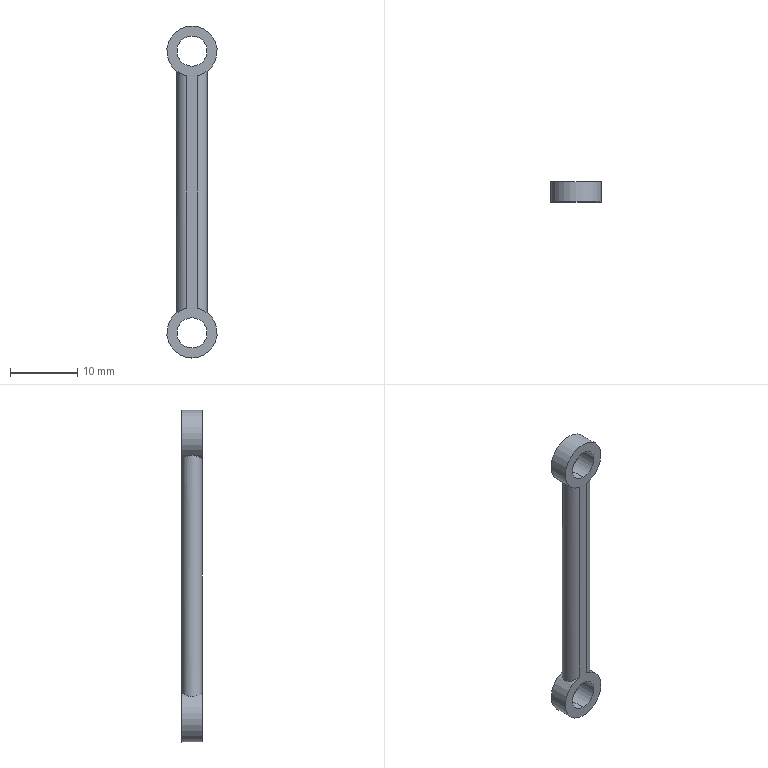Part | SolidWorks | features BaseBody 1, HoleWzd 1, Scale 1 | 1 solid | 12 faces | box 7.5 x 3 x 49.5 mm | volume 573.12 mm3 | cylinder 10 | plane 2 | commonest cylinder face diameters 4.5 x4 3 x3 7.5 x3
STEP:
#1=CARTESIAN_POINT('',(2.25,3.,44.25));
#2=VERTEX_POINT('',#1);
#3=CARTESIAN_POINT('',(2.25,3.,39.75));
#4=VERTEX_POINT('',#3);
#5=CARTESIAN_POINT('',(2.25,3.,42.));
#6=DIRECTION('',(0.,-1.,0.));
#7=DIRECTION('',(0.,0.,-1.));
#8=AXIS2_PLACEMENT_3D('',#5,#6,#7);
#9=CIRCLE('',#8,2.25);
#10=EDGE_CURVE('',#2,#4,#9,.T.);
#11=ORIENTED_EDGE('',*,*,#10,.F.);
#12=CARTESIAN_POINT('',(2.25,0.,44.25));
#13=VERTEX_POINT('',#12);
#14=CARTESIAN_POINT('',(2.25,0.,44.25));
#15=DIRECTION('',(0.,-1.,0.));
#16=VECTOR('',#15,1000.);
#17=LINE('',#14,#16);
#18=EDGE_CURVE('',#2,#13,#17,.T.);
#19=ORIENTED_EDGE('',*,*,#18,.T.);
#20=CARTESIAN_POINT('',(2.25,0.,39.75));
#21=VERTEX_POINT('',#20);
#22=CARTESIAN_POINT('',(2.25,0.,42.));
#23=DIRECTION('',(0.,-1.,0.));
#24=DIRECTION('',(0.,0.,-1.));
#25=AXIS2_PLACEMENT_3D('',#22,#23,#24);
#26=CIRCLE('',#25,2.25);
#27=EDGE_CURVE('',#13,#21,#26,.T.);
#28=ORIENTED_EDGE('',*,*,#27,.T.);
#29=CARTESIAN_POINT('',(2.25,0.,39.75));
#30=DIRECTION('',(0.,-1.,0.));
#31=VECTOR('',#30,1000.);
#32=LINE('',#29,#31);
#33=EDGE_CURVE('',#4,#21,#32,.T.);
#34=ORIENTED_EDGE('',*,*,#33,.F.);
#35=EDGE_LOOP('',(#11,#19,#28,#34));
#36=FACE_OUTER_BOUND('',#35,.T.);
#37=CARTESIAN_POINT('',(2.25,0.,42.));
#38=DIRECTION('',(0.,-1.,0.));
#39=DIRECTION('',(0.,0.,-1.));
#40=AXIS2_PLACEMENT_3D('',#37,#38,#39);
#41=CYLINDRICAL_SURFACE('',#40,2.25);
#42=ADVANCED_FACE('',(#36),#41,.F.);
#43=CARTESIAN_POINT('',(2.25,3.,2.25));
#44=VERTEX_POINT('',#43);
#45=CARTESIAN_POINT('',(2.25,3.,-2.25));
#46=VERTEX_POINT('',#45);
#47=CARTESIAN_POINT('',(2.25,3.,0.));
#48=DIRECTION('',(0.,-1.,0.));
#49=DIRECTION('',(0.,0.,-1.));
#50=AXIS2_PLACEMENT_3D('',#47,#48,#49);
#51=CIRCLE('',#50,2.25);
#52=EDGE_CURVE('',#44,#46,#51,.T.);
#53=ORIENTED_EDGE('',*,*,#52,.F.);
#54=CARTESIAN_POINT('',(2.25,0.,2.25));
#55=VERTEX_POINT('',#54);
#56=CARTESIAN_POINT('',(2.25,0.,2.25));
#57=DIRECTION('',(0.,-1.,0.));
#58=VECTOR('',#57,1000.);
#59=LINE('',#56,#58);
#60=EDGE_CURVE('',#44,#55,#59,.T.);
#61=ORIENTED_EDGE('',*,*,#60,.T.);
#62=CARTESIAN_POINT('',(2.25,0.,-2.25));
#63=VERTEX_POINT('',#62);
#64=CARTESIAN_POINT('',(2.25,0.,0.));
#65=DIRECTION('',(0.,-1.,0.));
#66=DIRECTION('',(0.,0.,-1.));
#67=AXIS2_PLACEMENT_3D('',#64,#65,#66);
#68=CIRCLE('',#67,2.25);
#69=EDGE_CURVE('',#55,#63,#68,.T.);
#70=ORIENTED_EDGE('',*,*,#69,.T.);
#71=CARTESIAN_POINT('',(2.25,0.,-2.25));
#72=DIRECTION('',(0.,-1.,0.));
#73=VECTOR('',#72,1000.);
#74=LINE('',#71,#73);
#75=EDGE_CURVE('',#46,#63,#74,.T.);
#76=ORIENTED_EDGE('',*,*,#75,.F.);
#77=EDGE_LOOP('',(#53,#61,#70,#76));
#78=FACE_OUTER_BOUND('',#77,.T.);
#79=CARTESIAN_POINT('',(2.25,0.,0.));
#80=DIRECTION('',(0.,-1.,0.));
#81=DIRECTION('',(0.,0.,-1.));
#82=AXIS2_PLACEMENT_3D('',#79,#80,#81);
#83=CYLINDRICAL_SURFACE('',#82,2.25);
#84=ADVANCED_FACE('',(#78),#83,.F.);
#85=CARTESIAN_POINT('',(3.,0.,3.674));
#86=VERTEX_POINT('',#85);
#87=CARTESIAN_POINT('',(4.5,1.5,3.));
#88=VERTEX_POINT('',#87);
#89=CARTESIAN_POINT('',(3.,0.,3.674));
#90=CARTESIAN_POINT('',(3.102,0.,3.654));
#91=CARTESIAN_POINT('',(3.2,0.0102,3.629));
#92=CARTESIAN_POINT('',(3.393,0.04905,3.573));
#93=CARTESIAN_POINT('',(3.488,0.07814,3.541));
#94=CARTESIAN_POINT('',(3.667,0.1528,3.473));
#95=CARTESIAN_POINT('',(3.751,0.1981,3.438));
#96=CARTESIAN_POINT('',(3.911,0.3041,3.363));
#97=CARTESIAN_POINT('',(3.986,0.3652,3.325));
#98=CARTESIAN_POINT('',(4.189,0.5659,3.213));
#99=CARTESIAN_POINT('',(4.301,0.728,3.141));
#100=CARTESIAN_POINT('',(4.418,1.,3.06));
#101=CARTESIAN_POINT('',(4.448,1.097,3.038));
#102=CARTESIAN_POINT('',(4.49,1.296,3.008));
#103=CARTESIAN_POINT('',(4.5,1.397,3.));
#104=CARTESIAN_POINT('',(4.5,1.5,3.));
#105=B_SPLINE_CURVE_WITH_KNOTS('',3,(#89,#90,#91,#92,#93,#94,#95,#96,#97,#98,#99,#100,#101,#102,#103,#104),.UNSPECIFIED.,.F.,.F.,(4,2,2,2,2,2,2,4),(0.,0.0003062,0.0006124,0.0009186,0.001225,0.001837,0.002143,0.00245),.UNSPECIFIED.);
#106=EDGE_CURVE('',#86,#88,#105,.T.);
#107=ORIENTED_EDGE('',*,*,#106,.T.);
#108=CARTESIAN_POINT('',(4.5,1.5,39.));
#109=VERTEX_POINT('',#108);
#110=CARTESIAN_POINT('',(4.5,1.5,0.));
#111=DIRECTION('',(0.,0.,1.));
#112=VECTOR('',#111,1000.);
#113=LINE('',#110,#112);
#114=EDGE_CURVE('',#88,#109,#113,.T.);
#115=ORIENTED_EDGE('',*,*,#114,.T.);
#116=CARTESIAN_POINT('',(3.,0.,38.326));
#117=VERTEX_POINT('',#116);
#118=CARTESIAN_POINT('',(4.5,1.5,39.));
#119=CARTESIAN_POINT('',(4.5,1.398,39.));
#120=CARTESIAN_POINT('',(4.489,1.294,38.992));
#121=CARTESIAN_POINT('',(4.448,1.096,38.962));
#122=CARTESIAN_POINT('',(4.417,0.9993,38.939));
#123=CARTESIAN_POINT('',(4.3,0.7262,38.859));
#124=CARTESIAN_POINT('',(4.188,0.5647,38.786));
#125=CARTESIAN_POINT('',(3.917,0.2975,38.637));
#126=CARTESIAN_POINT('',(3.755,0.1897,38.56));
#127=CARTESIAN_POINT('',(3.488,0.07846,38.459));
#128=CARTESIAN_POINT('',(3.394,0.04921,38.427));
#129=CARTESIAN_POINT('',(3.2,0.01017,38.371));
#130=CARTESIAN_POINT('',(3.101,0.,38.346));
#131=CARTESIAN_POINT('',(3.,0.,38.326));
#132=B_SPLINE_CURVE_WITH_KNOTS('',3,(#118,#119,#120,#121,#122,#123,#124,#125,#126,#127,#128,#129,#130,#131),.UNSPECIFIED.,.F.,.F.,(4,2,2,2,2,2,4),(0.00245,0.002755,0.00306,0.003671,0.004282,0.004588,0.004893),.UNSPECIFIED.);
#133=EDGE_CURVE('',#109,#117,#132,.T.);
#134=ORIENTED_EDGE('',*,*,#133,.T.);
#135=CARTESIAN_POINT('',(3.,0.,0.));
#136=DIRECTION('',(0.,0.,-1.));
#137=VECTOR('',#136,1000.);
#138=LINE('',#135,#137);
#139=EDGE_CURVE('',#117,#86,#138,.T.);
#140=ORIENTED_EDGE('',*,*,#139,.T.);
#141=EDGE_LOOP('',(#107,#115,#134,#140));
#142=FACE_OUTER_BOUND('',#141,.T.);
#143=CARTESIAN_POINT('',(3.,1.5,0.));
#144=DIRECTION('',(0.,0.,1.));
#145=DIRECTION('',(1.,0.,0.));
#146=AXIS2_PLACEMENT_3D('',#143,#144,#145);
#147=CYLINDRICAL_SURFACE('',#146,1.5);
#148=ADVANCED_FACE('',(#142),#147,.T.);
#149=CARTESIAN_POINT('',(1.5,3.,3.674));
#150=VERTEX_POINT('',#149);
#151=CARTESIAN_POINT('',(2.25,3.,-3.75));
#152=VERTEX_POINT('',#151);
#153=CARTESIAN_POINT('',(2.25,3.,0.));
#154=DIRECTION('',(0.,-1.,0.));
#155=DIRECTION('',(0.,0.,-1.));
#156=AXIS2_PLACEMENT_3D('',#153,#154,#155);
#157=CIRCLE('',#156,3.75);
#158=EDGE_CURVE('',#150,#152,#157,.T.);
#159=ORIENTED_EDGE('',*,*,#158,.T.);
#160=CARTESIAN_POINT('',(2.25,0.,-3.75));
#161=VERTEX_POINT('',#160);
#162=CARTESIAN_POINT('',(2.25,3.,-3.75));
#163=DIRECTION('',(0.,-1.,0.));
#164=VECTOR('',#163,1000.);
#165=LINE('',#162,#164);
#166=EDGE_CURVE('',#152,#161,#165,.T.);
#167=ORIENTED_EDGE('',*,*,#166,.T.);
#168=CARTESIAN_POINT('',(1.5,0.,3.674));
#169=VERTEX_POINT('',#168);
#170=CARTESIAN_POINT('',(2.25,0.,0.));
#171=DIRECTION('',(0.,1.,0.));
#172=DIRECTION('',(0.,0.,-1.));
#173=AXIS2_PLACEMENT_3D('',#170,#171,#172);
#174=CIRCLE('',#173,3.75);
#175=EDGE_CURVE('',#161,#169,#174,.T.);
#176=ORIENTED_EDGE('',*,*,#175,.T.);
#177=CARTESIAN_POINT('',(1.5,0.,3.674));
#178=CARTESIAN_POINT('',(1.399,0.,3.654));
#179=CARTESIAN_POINT('',(1.3,0.01018,3.629));
#180=CARTESIAN_POINT('',(1.108,0.04892,3.573));
#181=CARTESIAN_POINT('',(1.013,0.07794,3.541));
#182=CARTESIAN_POINT('',(0.834,0.1524,3.474));
#183=CARTESIAN_POINT('',(0.7497,0.1976,3.438));
#184=CARTESIAN_POINT('',(0.5905,0.3034,3.364));
#185=CARTESIAN_POINT('',(0.5154,0.3644,3.326));
#186=CARTESIAN_POINT('',(0.3121,0.5646,3.214));
#187=CARTESIAN_POINT('',(0.1999,0.7263,3.141));
#188=CARTESIAN_POINT('',(0.08309,0.9979,3.061));
#189=CARTESIAN_POINT('',(0.05223,1.095,3.039));
#190=CARTESIAN_POINT('',(0.0108,1.294,3.008));
#191=CARTESIAN_POINT('',(0.0002187,1.394,3.));
#192=CARTESIAN_POINT('',(-0.0002121,1.599,3.));
#193=CARTESIAN_POINT('',(0.01036,1.703,3.008));
#194=CARTESIAN_POINT('',(0.05114,1.901,3.038));
#195=CARTESIAN_POINT('',(0.08176,1.998,3.06));
#196=CARTESIAN_POINT('',(0.1988,2.272,3.141));
#197=CARTESIAN_POINT('',(0.3108,2.434,3.213));
#198=CARTESIAN_POINT('',(0.5824,2.702,3.362));
#199=CARTESIAN_POINT('',(0.744,2.81,3.44));
#200=CARTESIAN_POINT('',(1.011,2.921,3.541));
#201=CARTESIAN_POINT('',(1.106,2.951,3.573));
#202=CARTESIAN_POINT('',(1.299,2.99,3.629));
#203=CARTESIAN_POINT('',(1.398,3.,3.654));
#204=CARTESIAN_POINT('',(1.5,3.,3.674));
#205=B_SPLINE_CURVE_WITH_KNOTS('',3,(#177,#178,#179,#180,#181,#182,#183,#184,#185,#186,#187,#188,#189,#190,#191,#192,#193,#194,#195,#196,#197,#198,#199,#200,#201,#202,#203,#204),.UNSPECIFIED.,.F.,.F.,(4,2,2,2,2,2,2,2,2,2,2,2,2,4),(0.,0.0003058,0.0006116,0.0009174,0.001223,0.001835,0.002141,0.002446,0.002752,0.003058,0.00367,0.004281,0.004587,0.004893),.UNSPECIFIED.);
#206=EDGE_CURVE('',#169,#150,#205,.T.);
#207=ORIENTED_EDGE('',*,*,#206,.T.);
#208=EDGE_LOOP('',(#159,#167,#176,#207));
#209=FACE_OUTER_BOUND('',#208,.T.);
#210=CARTESIAN_POINT('',(2.25,3.,0.));
#211=DIRECTION('',(0.,-1.,0.));
#212=DIRECTION('',(0.,0.,-1.));
#213=AXIS2_PLACEMENT_3D('',#210,#211,#212);
#214=CYLINDRICAL_SURFACE('',#213,3.75);
#215=ADVANCED_FACE('',(#209),#214,.T.);
#216=ORIENTED_EDGE('',*,*,#114,.F.);
#217=CARTESIAN_POINT('',(3.,3.,3.674));
#218=VERTEX_POINT('',#217);
#219=CARTESIAN_POINT('',(4.5,1.5,3.));
#220=CARTESIAN_POINT('',(4.5,1.602,3.));
#221=CARTESIAN_POINT('',(4.489,1.706,3.008));
#222=CARTESIAN_POINT('',(4.448,1.904,3.038));
#223=CARTESIAN_POINT('',(4.417,2.001,3.061));
#224=CARTESIAN_POINT('',(4.3,2.274,3.141));
#225=CARTESIAN_POINT('',(4.188,2.435,3.214));
#226=CARTESIAN_POINT('',(3.917,2.703,3.363));
#227=CARTESIAN_POINT('',(3.755,2.81,3.44));
#228=CARTESIAN_POINT('',(3.488,2.922,3.541));
#229=CARTESIAN_POINT('',(3.394,2.951,3.573));
#230=CARTESIAN_POINT('',(3.2,2.99,3.629));
#231=CARTESIAN_POINT('',(3.101,3.,3.654));
#232=CARTESIAN_POINT('',(3.,3.,3.674));
#233=B_SPLINE_CURVE_WITH_KNOTS('',3,(#219,#220,#221,#222,#223,#224,#225,#226,#227,#228,#229,#230,#231,#232),.UNSPECIFIED.,.F.,.F.,(4,2,2,2,2,2,4),(0.00245,0.002755,0.00306,0.003671,0.004282,0.004588,0.004893),.UNSPECIFIED.);
#234=EDGE_CURVE('',#88,#218,#233,.T.);
#235=ORIENTED_EDGE('',*,*,#234,.T.);
#236=CARTESIAN_POINT('',(3.,3.,38.326));
#237=VERTEX_POINT('',#236);
#238=CARTESIAN_POINT('',(3.,3.,0.));
#239=DIRECTION('',(0.,0.,1.));
#240=VECTOR('',#239,1000.);
#241=LINE('',#238,#240);
#242=EDGE_CURVE('',#218,#237,#241,.T.);
#243=ORIENTED_EDGE('',*,*,#242,.T.);
#244=CARTESIAN_POINT('',(3.,3.,38.326));
#245=CARTESIAN_POINT('',(3.102,3.,38.346));
#246=CARTESIAN_POINT('',(3.2,2.99,38.371));
#247=CARTESIAN_POINT('',(3.393,2.951,38.427));
#248=CARTESIAN_POINT('',(3.488,2.922,38.459));
#249=CARTESIAN_POINT('',(3.667,2.847,38.527));
#250=CARTESIAN_POINT('',(3.751,2.802,38.562));
#251=CARTESIAN_POINT('',(3.911,2.696,38.637));
#252=CARTESIAN_POINT('',(3.986,2.635,38.675));
#253=CARTESIAN_POINT('',(4.189,2.434,38.787));
#254=CARTESIAN_POINT('',(4.301,2.272,38.859));
#255=CARTESIAN_POINT('',(4.418,2.,38.94));
#256=CARTESIAN_POINT('',(4.448,1.903,38.962));
#257=CARTESIAN_POINT('',(4.49,1.704,38.992));
#258=CARTESIAN_POINT('',(4.5,1.603,39.));
#259=CARTESIAN_POINT('',(4.5,1.5,39.));
#260=B_SPLINE_CURVE_WITH_KNOTS('',3,(#244,#245,#246,#247,#248,#249,#250,#251,#252,#253,#254,#255,#256,#257,#258,#259),.UNSPECIFIED.,.F.,.F.,(4,2,2,2,2,2,2,4),(0.,0.0003062,0.0006124,0.0009186,0.001225,0.001837,0.002143,0.00245),.UNSPECIFIED.);
#261=EDGE_CURVE('',#237,#109,#260,.T.);
#262=ORIENTED_EDGE('',*,*,#261,.T.);
#263=EDGE_LOOP('',(#216,#235,#243,#262));
#264=FACE_OUTER_BOUND('',#263,.T.);
#265=CARTESIAN_POINT('',(3.,1.5,0.));
#266=DIRECTION('',(0.,0.,1.));
#267=DIRECTION('',(1.,0.,0.));
#268=AXIS2_PLACEMENT_3D('',#265,#266,#267);
#269=CYLINDRICAL_SURFACE('',#268,1.5);
#270=ADVANCED_FACE('',(#264),#269,.T.);
#271=ORIENTED_EDGE('',*,*,#166,.F.);
#272=CARTESIAN_POINT('',(2.25,3.,0.));
#273=DIRECTION('',(0.,-1.,0.));
#274=DIRECTION('',(0.,0.,-1.));
#275=AXIS2_PLACEMENT_3D('',#272,#273,#274);
#276=CIRCLE('',#275,3.75);
#277=EDGE_CURVE('',#152,#218,#276,.T.);
#278=ORIENTED_EDGE('',*,*,#277,.T.);
#279=ORIENTED_EDGE('',*,*,#234,.F.);
#280=ORIENTED_EDGE('',*,*,#106,.F.);
#281=CARTESIAN_POINT('',(2.25,0.,0.));
#282=DIRECTION('',(0.,1.,0.));
#283=DIRECTION('',(0.,0.,-1.));
#284=AXIS2_PLACEMENT_3D('',#281,#282,#283);
#285=CIRCLE('',#284,3.75);
#286=EDGE_CURVE('',#86,#161,#285,.T.);
#287=ORIENTED_EDGE('',*,*,#286,.T.);
#288=EDGE_LOOP('',(#271,#278,#279,#280,#287));
#289=FACE_OUTER_BOUND('',#288,.T.);
#290=CARTESIAN_POINT('',(2.25,3.,0.));
#291=DIRECTION('',(0.,-1.,0.));
#292=DIRECTION('',(0.,0.,-1.));
#293=AXIS2_PLACEMENT_3D('',#290,#291,#292);
#294=CYLINDRICAL_SURFACE('',#293,3.75);
#295=ADVANCED_FACE('',(#289),#294,.T.);
#296=CARTESIAN_POINT('',(2.25,0.,42.));
#297=DIRECTION('',(0.,-1.,0.));
#298=DIRECTION('',(0.,0.,-1.));
#299=AXIS2_PLACEMENT_3D('',#296,#297,#298);
#300=CIRCLE('',#299,2.25);
#301=EDGE_CURVE('',#21,#13,#300,.T.);
#302=ORIENTED_EDGE('',*,*,#301,.F.);
#303=ORIENTED_EDGE('',*,*,#27,.F.);
#304=EDGE_LOOP('',(#302,#303));
#305=FACE_BOUND('',#304,.T.);
#306=CARTESIAN_POINT('',(2.25,0.,0.));
#307=DIRECTION('',(0.,-1.,0.));
#308=DIRECTION('',(0.,0.,-1.));
#309=AXIS2_PLACEMENT_3D('',#306,#307,#308);
#310=CIRCLE('',#309,2.25);
#311=EDGE_CURVE('',#63,#55,#310,.T.);
#312=ORIENTED_EDGE('',*,*,#311,.F.);
#313=ORIENTED_EDGE('',*,*,#69,.F.);
#314=EDGE_LOOP('',(#312,#313));
#315=FACE_BOUND('',#314,.T.);
#316=CARTESIAN_POINT('',(1.5,0.,38.326));
#317=VERTEX_POINT('',#316);
#318=CARTESIAN_POINT('',(1.5,0.,0.));
#319=DIRECTION('',(0.,0.,-1.));
#320=VECTOR('',#319,1000.);
#321=LINE('',#318,#320);
#322=EDGE_CURVE('',#317,#169,#321,.T.);
#323=ORIENTED_EDGE('',*,*,#322,.T.);
#324=ORIENTED_EDGE('',*,*,#175,.F.);
#325=ORIENTED_EDGE('',*,*,#286,.F.);
#326=ORIENTED_EDGE('',*,*,#139,.F.);
#327=CARTESIAN_POINT('',(2.25,0.,42.));
#328=DIRECTION('',(0.,-1.,0.));
#329=DIRECTION('',(0.,0.,-1.));
#330=AXIS2_PLACEMENT_3D('',#327,#328,#329);
#331=CIRCLE('',#330,3.75);
#332=EDGE_CURVE('',#117,#317,#331,.T.);
#333=ORIENTED_EDGE('',*,*,#332,.T.);
#334=EDGE_LOOP('',(#323,#324,#325,#326,#333));
#335=FACE_OUTER_BOUND('',#334,.T.);
#336=CARTESIAN_POINT('',(2.25,0.,0.));
#337=DIRECTION('',(0.,-1.,0.));
#338=DIRECTION('',(0.,0.,-1.));
#339=AXIS2_PLACEMENT_3D('',#336,#337,#338);
#340=PLANE('',#339);
#341=ADVANCED_FACE('',(#305,#315,#335),#340,.T.);
#342=ORIENTED_EDGE('',*,*,#332,.F.);
#343=ORIENTED_EDGE('',*,*,#133,.F.);
#344=ORIENTED_EDGE('',*,*,#261,.F.);
#345=CARTESIAN_POINT('',(1.5,3.,38.326));
#346=VERTEX_POINT('',#345);
#347=CARTESIAN_POINT('',(2.25,3.,42.));
#348=DIRECTION('',(0.,-1.,0.));
#349=DIRECTION('',(0.,0.,-1.));
#350=AXIS2_PLACEMENT_3D('',#347,#348,#349);
#351=CIRCLE('',#350,3.75);
#352=EDGE_CURVE('',#237,#346,#351,.T.);
#353=ORIENTED_EDGE('',*,*,#352,.T.);
#354=CARTESIAN_POINT('',(1.5,3.,38.326));
#355=CARTESIAN_POINT('',(1.399,3.,38.346));
#356=CARTESIAN_POINT('',(1.3,2.99,38.371));
#357=CARTESIAN_POINT('',(1.108,2.951,38.427));
#358=CARTESIAN_POINT('',(1.013,2.922,38.459));
#359=CARTESIAN_POINT('',(0.834,2.848,38.526));
#360=CARTESIAN_POINT('',(0.7497,2.802,38.562));
#361=CARTESIAN_POINT('',(0.5905,2.697,38.636));
#362=CARTESIAN_POINT('',(0.5154,2.636,38.674));
#363=CARTESIAN_POINT('',(0.3121,2.435,38.786));
#364=CARTESIAN_POINT('',(0.1999,2.274,38.859));
#365=CARTESIAN_POINT('',(0.08309,2.002,38.939));
#366=CARTESIAN_POINT('',(0.05223,1.905,38.961));
#367=CARTESIAN_POINT('',(0.0108,1.706,38.992));
#368=CARTESIAN_POINT('',(0.0002187,1.606,39.));
#369=CARTESIAN_POINT('',(-0.0002121,1.401,39.));
#370=CARTESIAN_POINT('',(0.01036,1.297,38.992));
#371=CARTESIAN_POINT('',(0.05114,1.099,38.962));
#372=CARTESIAN_POINT('',(0.08176,1.002,38.94));
#373=CARTESIAN_POINT('',(0.1988,0.7279,38.859));
#374=CARTESIAN_POINT('',(0.3108,0.5661,38.787));
#375=CARTESIAN_POINT('',(0.5824,0.2982,38.638));
#376=CARTESIAN_POINT('',(0.744,0.1902,38.56));
#377=CARTESIAN_POINT('',(1.011,0.07866,38.459));
#378=CARTESIAN_POINT('',(1.106,0.04934,38.427));
#379=CARTESIAN_POINT('',(1.299,0.0102,38.371));
#380=CARTESIAN_POINT('',(1.398,0.,38.346));
#381=CARTESIAN_POINT('',(1.5,0.,38.326));
#382=B_SPLINE_CURVE_WITH_KNOTS('',3,(#354,#355,#356,#357,#358,#359,#360,#361,#362,#363,#364,#365,#366,#367,#368,#369,#370,#371,#372,#373,#374,#375,#376,#377,#378,#379,#380,#381),.UNSPECIFIED.,.F.,.F.,(4,2,2,2,2,2,2,2,2,2,2,2,2,4),(0.,0.0003058,0.0006116,0.0009174,0.001223,0.001835,0.002141,0.002446,0.002752,0.003058,0.00367,0.004281,0.004587,0.004893),.UNSPECIFIED.);
#383=EDGE_CURVE('',#346,#317,#382,.T.);
#384=ORIENTED_EDGE('',*,*,#383,.T.);
#385=EDGE_LOOP('',(#342,#343,#344,#353,#384));
#386=FACE_OUTER_BOUND('',#385,.T.);
#387=CARTESIAN_POINT('',(2.25,3.,42.));
#388=DIRECTION('',(0.,-1.,0.));
#389=DIRECTION('',(0.,0.,-1.));
#390=AXIS2_PLACEMENT_3D('',#387,#388,#389);
#391=CYLINDRICAL_SURFACE('',#390,3.75);
#392=ADVANCED_FACE('',(#386),#391,.T.);
#393=CARTESIAN_POINT('',(2.25,3.,42.));
#394=DIRECTION('',(0.,-1.,0.));
#395=DIRECTION('',(0.,0.,-1.));
#396=AXIS2_PLACEMENT_3D('',#393,#394,#395);
#397=CIRCLE('',#396,2.25);
#398=EDGE_CURVE('',#4,#2,#397,.T.);
#399=ORIENTED_EDGE('',*,*,#398,.T.);
#400=ORIENTED_EDGE('',*,*,#10,.T.);
#401=EDGE_LOOP('',(#399,#400));
#402=FACE_BOUND('',#401,.T.);
#403=CARTESIAN_POINT('',(2.25,3.,0.));
#404=DIRECTION('',(0.,-1.,0.));
#405=DIRECTION('',(0.,0.,-1.));
#406=AXIS2_PLACEMENT_3D('',#403,#404,#405);
#407=CIRCLE('',#406,2.25);
#408=EDGE_CURVE('',#46,#44,#407,.T.);
#409=ORIENTED_EDGE('',*,*,#408,.T.);
#410=ORIENTED_EDGE('',*,*,#52,.T.);
#411=EDGE_LOOP('',(#409,#410));
#412=FACE_BOUND('',#411,.T.);
#413=ORIENTED_EDGE('',*,*,#158,.F.);
#414=CARTESIAN_POINT('',(1.5,3.,0.));
#415=DIRECTION('',(0.,0.,1.));
#416=VECTOR('',#415,1000.);
#417=LINE('',#414,#416);
#418=EDGE_CURVE('',#150,#346,#417,.T.);
#419=ORIENTED_EDGE('',*,*,#418,.T.);
#420=ORIENTED_EDGE('',*,*,#352,.F.);
#421=ORIENTED_EDGE('',*,*,#242,.F.);
#422=ORIENTED_EDGE('',*,*,#277,.F.);
#423=EDGE_LOOP('',(#413,#419,#420,#421,#422));
#424=FACE_OUTER_BOUND('',#423,.T.);
#425=CARTESIAN_POINT('',(2.25,3.,0.));
#426=DIRECTION('',(0.,1.,0.));
#427=DIRECTION('',(0.,0.,1.));
#428=AXIS2_PLACEMENT_3D('',#425,#426,#427);
#429=PLANE('',#428);
#430=ADVANCED_FACE('',(#402,#412,#424),#429,.T.);
#431=ORIENTED_EDGE('',*,*,#322,.F.);
#432=ORIENTED_EDGE('',*,*,#383,.F.);
#433=ORIENTED_EDGE('',*,*,#418,.F.);
#434=ORIENTED_EDGE('',*,*,#206,.F.);
#435=EDGE_LOOP('',(#431,#432,#433,#434));
#436=FACE_OUTER_BOUND('',#435,.T.);
#437=CARTESIAN_POINT('',(1.5,1.5,0.));
#438=DIRECTION('',(0.,0.,1.));
#439=DIRECTION('',(1.,0.,0.));
#440=AXIS2_PLACEMENT_3D('',#437,#438,#439);
#441=CYLINDRICAL_SURFACE('',#440,1.5);
#442=ADVANCED_FACE('',(#436),#441,.T.);
#443=ORIENTED_EDGE('',*,*,#60,.F.);
#444=ORIENTED_EDGE('',*,*,#408,.F.);
#445=ORIENTED_EDGE('',*,*,#75,.T.);
#446=ORIENTED_EDGE('',*,*,#311,.T.);
#447=EDGE_LOOP('',(#443,#444,#445,#446));
#448=FACE_OUTER_BOUND('',#447,.T.);
#449=CARTESIAN_POINT('',(2.25,0.,0.));
#450=DIRECTION('',(0.,-1.,0.));
#451=DIRECTION('',(0.,0.,-1.));
#452=AXIS2_PLACEMENT_3D('',#449,#450,#451);
#453=CYLINDRICAL_SURFACE('',#452,2.25);
#454=ADVANCED_FACE('',(#448),#453,.F.);
#455=ORIENTED_EDGE('',*,*,#18,.F.);
#456=ORIENTED_EDGE('',*,*,#398,.F.);
#457=ORIENTED_EDGE('',*,*,#33,.T.);
#458=ORIENTED_EDGE('',*,*,#301,.T.);
#459=EDGE_LOOP('',(#455,#456,#457,#458));
#460=FACE_OUTER_BOUND('',#459,.T.);
#461=CARTESIAN_POINT('',(2.25,0.,42.));
#462=DIRECTION('',(0.,-1.,0.));
#463=DIRECTION('',(0.,0.,-1.));
#464=AXIS2_PLACEMENT_3D('',#461,#462,#463);
#465=CYLINDRICAL_SURFACE('',#464,2.25);
#466=ADVANCED_FACE('',(#460),#465,.F.);
#467=CLOSED_SHELL('',(#42,#84,#148,#215,#270,#295,#341,#392,#430,#442,#454,#466));
#468=MANIFOLD_SOLID_BREP('',#467);
#469=CARTESIAN_POINT('',(0.,0.,0.));
#470=DIRECTION('',(0.,0.,1.));
#471=DIRECTION('',(1.,0.,0.));
#472=AXIS2_PLACEMENT_3D('',#469,#470,#471);
#473=(LENGTH_UNIT()NAMED_UNIT(*)SI_UNIT(.MILLI.,.METRE.));
#474=UNCERTAINTY_MEASURE_WITH_UNIT(LENGTH_MEASURE(0.00001),#473,'','');
#475=(NAMED_UNIT(*)PLANE_ANGLE_UNIT()SI_UNIT($,.RADIAN.));
#476=(NAMED_UNIT(*)SI_UNIT($,.STERADIAN.)SOLID_ANGLE_UNIT());
#477=(GEOMETRIC_REPRESENTATION_CONTEXT(3)GLOBAL_UNCERTAINTY_ASSIGNED_CONTEXT((#474))GLOBAL_UNIT_ASSIGNED_CONTEXT((#473,#475,#476))REPRESENTATION_CONTEXT('',''));
#478=ADVANCED_BREP_SHAPE_REPRESENTATION('',(#468,#472),#477);